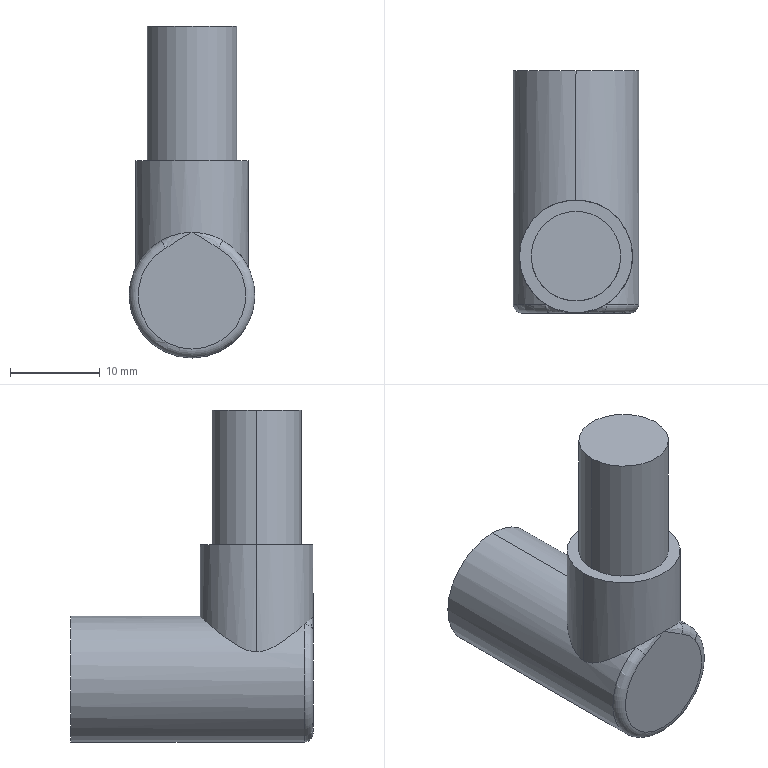Part | STEP file | Wire connector | 1 solid | 13 faces | box 14 x 27 x 37 mm | volume 6425 mm3 | cylinder 6 | plane 4 | spline 2 | torus 1 | commonest cylinder face diameters 10 x2 12.6 x2 14 x2